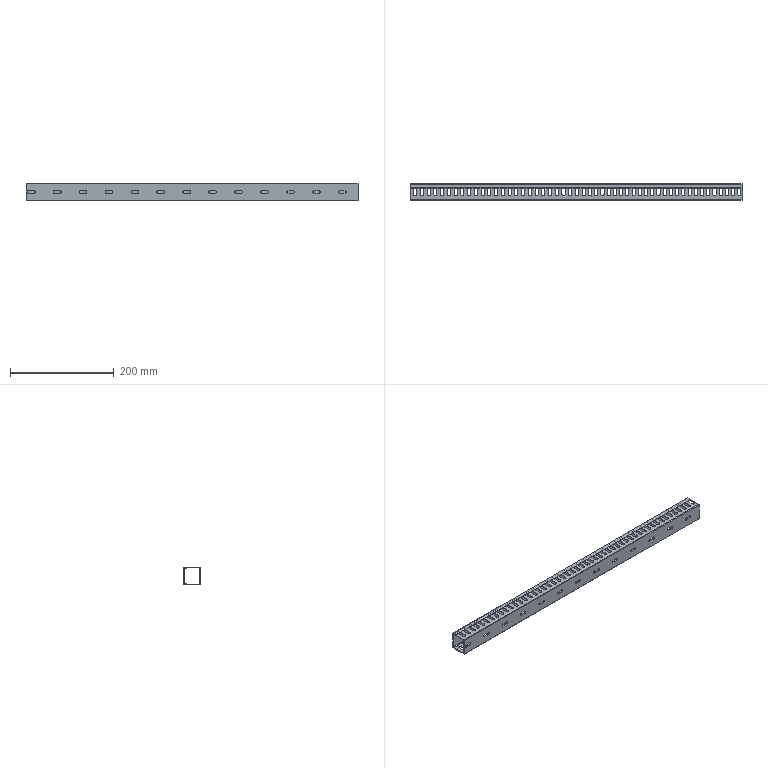Part | SolidWorks | features BaseBody 2 | 2 solids | 908 faces | box 640 x 31.5 x 34 mm | volume 111904 mm3 | plane 772 | cylinder 136 | commonest cylinder face diameters 6 x102 5 x26 1 x4 0.2 x2 2 x2